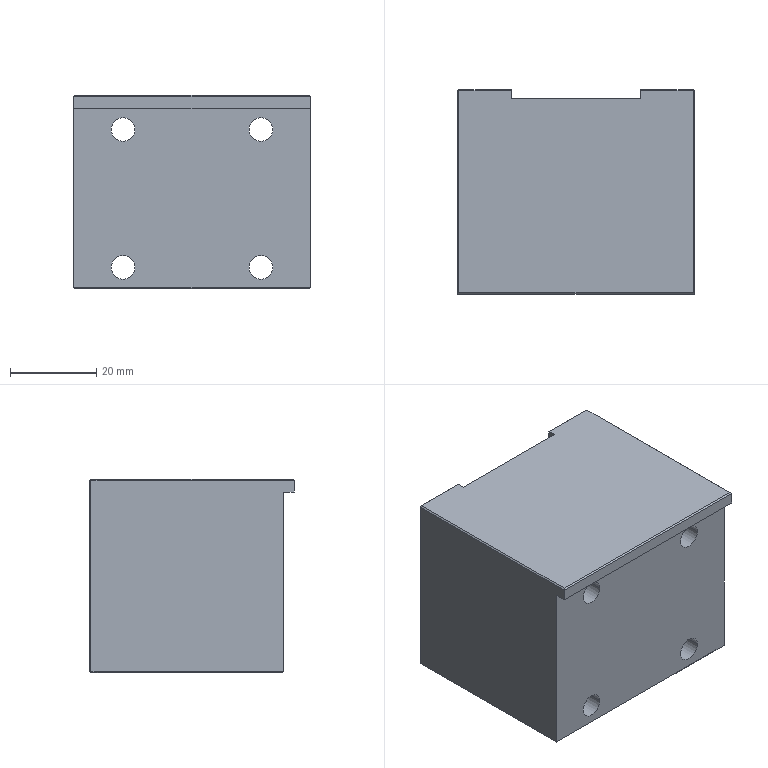Part | NX | 1 solid | 82 faces | box 55 x 47.5 x 45 mm | volume 102326 mm3 | plane 34 | cylinder 32 | cone 16 | commonest cylinder face diameters 2.5 x8 5 x8 5.5 x8 9.5 x8